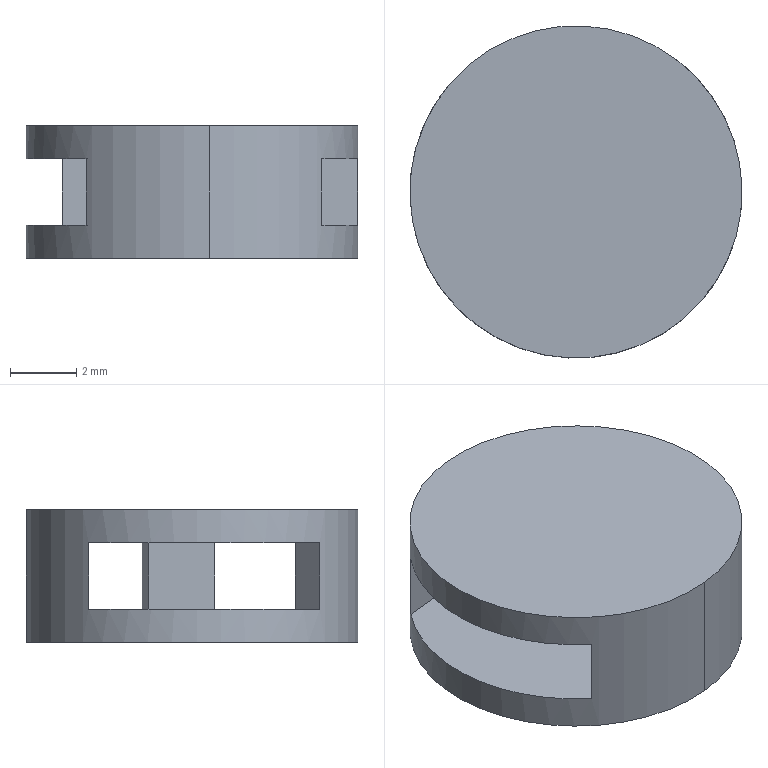Part | SolidWorks | features BaseBody 1 | 1 solid | 11 faces | box 10 x 10 x 4 mm | volume 194.495 mm3 | plane 9 | cylinder 2 | commonest cylinder face diameters 10 x2
STEP:
#1=CARTESIAN_POINT('',(349.672,130.094,60.5));
#2=VERTEX_POINT('',#1);
#3=CARTESIAN_POINT('',(349.672,130.094,62.5));
#4=VERTEX_POINT('',#3);
#5=CARTESIAN_POINT('',(349.672,130.094,63.5));
#6=DIRECTION('',(0.,0.,1.));
#7=VECTOR('',#6,1000.);
#8=LINE('',#5,#7);
#9=EDGE_CURVE('',#2,#4,#8,.T.);
#10=ORIENTED_EDGE('',*,*,#9,.T.);
#11=CARTESIAN_POINT('',(350.393,123.132,62.5));
#12=VERTEX_POINT('',#11);
#13=CARTESIAN_POINT('',(353.585,126.98,62.5));
#14=DIRECTION('',(0.,0.,1.));
#15=DIRECTION('',(-0.1029,0.9947,0.));
#16=AXIS2_PLACEMENT_3D('',#13,#14,#15);
#17=CIRCLE('',#16,5.);
#18=EDGE_CURVE('',#4,#12,#17,.T.);
#19=ORIENTED_EDGE('',*,*,#18,.T.);
#20=CARTESIAN_POINT('',(350.393,123.132,60.5));
#21=VERTEX_POINT('',#20);
#22=CARTESIAN_POINT('',(350.393,123.132,63.5));
#23=DIRECTION('',(0.,0.,-1.));
#24=VECTOR('',#23,1000.);
#25=LINE('',#22,#24);
#26=EDGE_CURVE('',#12,#21,#25,.T.);
#27=ORIENTED_EDGE('',*,*,#26,.T.);
#28=CARTESIAN_POINT('',(353.585,126.98,60.5));
#29=DIRECTION('',(0.,0.,-1.));
#30=DIRECTION('',(0.1029,-0.9947,0.));
#31=AXIS2_PLACEMENT_3D('',#28,#29,#30);
#32=CIRCLE('',#31,5.);
#33=EDGE_CURVE('',#21,#2,#32,.T.);
#34=ORIENTED_EDGE('',*,*,#33,.T.);
#35=EDGE_LOOP('',(#10,#19,#27,#34));
#36=FACE_BOUND('',#35,.T.);
#37=CARTESIAN_POINT('',(353.07,131.954,63.5));
#38=VERTEX_POINT('',#37);
#39=CARTESIAN_POINT('',(354.099,122.007,63.5));
#40=VERTEX_POINT('',#39);
#41=CARTESIAN_POINT('',(353.585,126.98,63.5));
#42=DIRECTION('',(0.,0.,1.));
#43=DIRECTION('',(-0.1029,0.9947,0.));
#44=AXIS2_PLACEMENT_3D('',#41,#42,#43);
#45=CIRCLE('',#44,5.);
#46=EDGE_CURVE('',#38,#40,#45,.T.);
#47=ORIENTED_EDGE('',*,*,#46,.F.);
#48=CARTESIAN_POINT('',(353.07,131.954,59.5));
#49=VERTEX_POINT('',#48);
#50=CARTESIAN_POINT('',(353.07,131.954,63.5));
#51=DIRECTION('',(0.,0.,-1.));
#52=VECTOR('',#51,1000.);
#53=LINE('',#50,#52);
#54=EDGE_CURVE('',#38,#49,#53,.T.);
#55=ORIENTED_EDGE('',*,*,#54,.T.);
#56=CARTESIAN_POINT('',(354.099,122.007,59.5));
#57=VERTEX_POINT('',#56);
#58=CARTESIAN_POINT('',(353.585,126.98,59.5));
#59=DIRECTION('',(0.,0.,1.));
#60=DIRECTION('',(-0.1029,0.9947,0.));
#61=AXIS2_PLACEMENT_3D('',#58,#59,#60);
#62=CIRCLE('',#61,5.);
#63=EDGE_CURVE('',#49,#57,#62,.T.);
#64=ORIENTED_EDGE('',*,*,#63,.T.);
#65=CARTESIAN_POINT('',(354.099,122.007,63.5));
#66=DIRECTION('',(0.,0.,-1.));
#67=VECTOR('',#66,1000.);
#68=LINE('',#65,#67);
#69=EDGE_CURVE('',#40,#57,#68,.T.);
#70=ORIENTED_EDGE('',*,*,#69,.F.);
#71=EDGE_LOOP('',(#47,#55,#64,#70));
#72=FACE_OUTER_BOUND('',#71,.T.);
#73=CARTESIAN_POINT('',(353.585,126.98,63.5));
#74=DIRECTION('',(0.,0.,-1.));
#75=DIRECTION('',(0.1029,-0.9947,0.));
#76=AXIS2_PLACEMENT_3D('',#73,#74,#75);
#77=CYLINDRICAL_SURFACE('',#76,5.);
#78=ADVANCED_FACE('',(#36,#72),#77,.T.);
#79=ORIENTED_EDGE('',*,*,#54,.F.);
#80=CARTESIAN_POINT('',(353.585,126.98,63.5));
#81=DIRECTION('',(0.,0.,1.));
#82=DIRECTION('',(-0.1029,0.9947,0.));
#83=AXIS2_PLACEMENT_3D('',#80,#81,#82);
#84=CIRCLE('',#83,5.);
#85=EDGE_CURVE('',#40,#38,#84,.T.);
#86=ORIENTED_EDGE('',*,*,#85,.F.);
#87=ORIENTED_EDGE('',*,*,#69,.T.);
#88=CARTESIAN_POINT('',(353.585,126.98,59.5));
#89=DIRECTION('',(0.,0.,1.));
#90=DIRECTION('',(-0.1029,0.9947,0.));
#91=AXIS2_PLACEMENT_3D('',#88,#89,#90);
#92=CIRCLE('',#91,5.);
#93=EDGE_CURVE('',#57,#49,#92,.T.);
#94=ORIENTED_EDGE('',*,*,#93,.T.);
#95=EDGE_LOOP('',(#79,#86,#87,#94));
#96=FACE_OUTER_BOUND('',#95,.T.);
#97=CARTESIAN_POINT('',(358.56,126.49,60.5));
#98=VERTEX_POINT('',#97);
#99=CARTESIAN_POINT('',(357.497,123.867,60.5));
#100=VERTEX_POINT('',#99);
#101=CARTESIAN_POINT('',(353.585,126.98,60.5));
#102=DIRECTION('',(0.,0.,-1.));
#103=DIRECTION('',(0.1029,-0.9947,0.));
#104=AXIS2_PLACEMENT_3D('',#101,#102,#103);
#105=CIRCLE('',#104,5.);
#106=EDGE_CURVE('',#98,#100,#105,.T.);
#107=ORIENTED_EDGE('',*,*,#106,.T.);
#108=CARTESIAN_POINT('',(357.497,123.867,62.5));
#109=VERTEX_POINT('',#108);
#110=CARTESIAN_POINT('',(357.497,123.867,63.5));
#111=DIRECTION('',(0.,0.,1.));
#112=VECTOR('',#111,1000.);
#113=LINE('',#110,#112);
#114=EDGE_CURVE('',#100,#109,#113,.T.);
#115=ORIENTED_EDGE('',*,*,#114,.T.);
#116=CARTESIAN_POINT('',(358.56,126.49,62.5));
#117=VERTEX_POINT('',#116);
#118=CARTESIAN_POINT('',(353.585,126.98,62.5));
#119=DIRECTION('',(0.,0.,1.));
#120=DIRECTION('',(-0.1029,0.9947,0.));
#121=AXIS2_PLACEMENT_3D('',#118,#119,#120);
#122=CIRCLE('',#121,5.);
#123=EDGE_CURVE('',#109,#117,#122,.T.);
#124=ORIENTED_EDGE('',*,*,#123,.T.);
#125=CARTESIAN_POINT('',(358.56,126.49,63.5));
#126=DIRECTION('',(0.,0.,-1.));
#127=VECTOR('',#126,1000.);
#128=LINE('',#125,#127);
#129=EDGE_CURVE('',#117,#98,#128,.T.);
#130=ORIENTED_EDGE('',*,*,#129,.T.);
#131=EDGE_LOOP('',(#107,#115,#124,#130));
#132=FACE_BOUND('',#131,.T.);
#133=CARTESIAN_POINT('',(358.355,128.479,62.5));
#134=VERTEX_POINT('',#133);
#135=CARTESIAN_POINT('',(356.776,130.829,62.5));
#136=VERTEX_POINT('',#135);
#137=CARTESIAN_POINT('',(353.585,126.98,62.5));
#138=DIRECTION('',(0.,0.,1.));
#139=DIRECTION('',(-0.1029,0.9947,0.));
#140=AXIS2_PLACEMENT_3D('',#137,#138,#139);
#141=CIRCLE('',#140,5.);
#142=EDGE_CURVE('',#134,#136,#141,.T.);
#143=ORIENTED_EDGE('',*,*,#142,.T.);
#144=CARTESIAN_POINT('',(356.776,130.829,60.5));
#145=VERTEX_POINT('',#144);
#146=CARTESIAN_POINT('',(356.776,130.829,63.5));
#147=DIRECTION('',(0.,0.,-1.));
#148=VECTOR('',#147,1000.);
#149=LINE('',#146,#148);
#150=EDGE_CURVE('',#136,#145,#149,.T.);
#151=ORIENTED_EDGE('',*,*,#150,.T.);
#152=CARTESIAN_POINT('',(358.355,128.479,60.5));
#153=VERTEX_POINT('',#152);
#154=CARTESIAN_POINT('',(353.585,126.98,60.5));
#155=DIRECTION('',(0.,0.,-1.));
#156=DIRECTION('',(0.1029,-0.9947,0.));
#157=AXIS2_PLACEMENT_3D('',#154,#155,#156);
#158=CIRCLE('',#157,5.);
#159=EDGE_CURVE('',#145,#153,#158,.T.);
#160=ORIENTED_EDGE('',*,*,#159,.T.);
#161=CARTESIAN_POINT('',(358.355,128.479,63.5));
#162=DIRECTION('',(0.,0.,1.));
#163=VECTOR('',#162,1000.);
#164=LINE('',#161,#163);
#165=EDGE_CURVE('',#153,#134,#164,.T.);
#166=ORIENTED_EDGE('',*,*,#165,.T.);
#167=EDGE_LOOP('',(#143,#151,#160,#166));
#168=FACE_BOUND('',#167,.T.);
#169=CARTESIAN_POINT('',(353.585,126.98,63.5));
#170=DIRECTION('',(0.,0.,-1.));
#171=DIRECTION('',(0.1029,-0.9947,0.));
#172=AXIS2_PLACEMENT_3D('',#169,#170,#171);
#173=CYLINDRICAL_SURFACE('',#172,5.);
#174=ADVANCED_FACE('',(#96,#132,#168),#173,.T.);
#175=ORIENTED_EDGE('',*,*,#85,.T.);
#176=ORIENTED_EDGE('',*,*,#46,.T.);
#177=EDGE_LOOP('',(#175,#176));
#178=FACE_OUTER_BOUND('',#177,.T.);
#179=CARTESIAN_POINT('',(353.585,126.98,63.5));
#180=DIRECTION('',(0.,0.,1.));
#181=DIRECTION('',(-0.1029,0.9947,0.));
#182=AXIS2_PLACEMENT_3D('',#179,#180,#181);
#183=PLANE('',#182);
#184=ADVANCED_FACE('',(#178),#183,.T.);
#185=ORIENTED_EDGE('',*,*,#93,.F.);
#186=ORIENTED_EDGE('',*,*,#63,.F.);
#187=EDGE_LOOP('',(#185,#186));
#188=FACE_OUTER_BOUND('',#187,.T.);
#189=CARTESIAN_POINT('',(353.585,126.98,59.5));
#190=DIRECTION('',(0.,0.,1.));
#191=DIRECTION('',(-0.1029,0.9947,0.));
#192=AXIS2_PLACEMENT_3D('',#189,#190,#191);
#193=PLANE('',#192);
#194=ADVANCED_FACE('',(#188),#193,.F.);
#195=CARTESIAN_POINT('',(356.929,123.808,62.5));
#196=DIRECTION('',(-0.9947,-0.1029,0.));
#197=VECTOR('',#196,1000.);
#198=LINE('',#195,#197);
#199=EDGE_CURVE('',#109,#12,#198,.T.);
#200=ORIENTED_EDGE('',*,*,#199,.F.);
#201=ORIENTED_EDGE('',*,*,#114,.F.);
#202=CARTESIAN_POINT('',(356.929,123.808,60.5));
#203=DIRECTION('',(-0.9947,-0.1029,0.));
#204=VECTOR('',#203,1000.);
#205=LINE('',#202,#204);
#206=EDGE_CURVE('',#100,#21,#205,.T.);
#207=ORIENTED_EDGE('',*,*,#206,.T.);
#208=ORIENTED_EDGE('',*,*,#26,.F.);
#209=EDGE_LOOP('',(#200,#201,#207,#208));
#210=FACE_OUTER_BOUND('',#209,.T.);
#211=CARTESIAN_POINT('',(356.929,123.808,60.5));
#212=DIRECTION('',(0.1029,-0.9947,0.));
#213=DIRECTION('',(0.,0.,1.));
#214=AXIS2_PLACEMENT_3D('',#211,#212,#213);
#215=PLANE('',#214);
#216=ADVANCED_FACE('',(#210),#215,.F.);
#217=ORIENTED_EDGE('',*,*,#206,.F.);
#218=ORIENTED_EDGE('',*,*,#106,.F.);
#219=CARTESIAN_POINT('',(356.672,126.295,60.5));
#220=VERTEX_POINT('',#219);
#221=CARTESIAN_POINT('',(358.661,126.5,60.5));
#222=DIRECTION('',(-0.9947,-0.1029,0.));
#223=VECTOR('',#222,1000.);
#224=LINE('',#221,#223);
#225=EDGE_CURVE('',#98,#220,#224,.T.);
#226=ORIENTED_EDGE('',*,*,#225,.T.);
#227=CARTESIAN_POINT('',(356.466,128.284,60.5));
#228=VERTEX_POINT('',#227);
#229=CARTESIAN_POINT('',(356.929,123.808,60.5));
#230=DIRECTION('',(0.1029,-0.9947,0.));
#231=VECTOR('',#230,1000.);
#232=LINE('',#229,#231);
#233=EDGE_CURVE('',#228,#220,#232,.T.);
#234=ORIENTED_EDGE('',*,*,#233,.F.);
#235=CARTESIAN_POINT('',(358.455,128.49,60.5));
#236=DIRECTION('',(-0.9947,-0.1029,0.));
#237=VECTOR('',#236,1000.);
#238=LINE('',#235,#237);
#239=EDGE_CURVE('',#153,#228,#238,.T.);
#240=ORIENTED_EDGE('',*,*,#239,.F.);
#241=ORIENTED_EDGE('',*,*,#159,.F.);
#242=CARTESIAN_POINT('',(356.208,130.771,60.5));
#243=DIRECTION('',(-0.9947,-0.1029,0.));
#244=VECTOR('',#243,1000.);
#245=LINE('',#242,#244);
#246=EDGE_CURVE('',#145,#2,#245,.T.);
#247=ORIENTED_EDGE('',*,*,#246,.T.);
#248=ORIENTED_EDGE('',*,*,#33,.F.);
#249=EDGE_LOOP('',(#217,#218,#226,#234,#240,#241,#247,#248));
#250=FACE_OUTER_BOUND('',#249,.T.);
#251=CARTESIAN_POINT('',(356.929,123.808,60.5));
#252=DIRECTION('',(0.,0.,-1.));
#253=DIRECTION('',(0.1029,-0.9947,0.));
#254=AXIS2_PLACEMENT_3D('',#251,#252,#253);
#255=PLANE('',#254);
#256=ADVANCED_FACE('',(#250),#255,.F.);
#257=ORIENTED_EDGE('',*,*,#246,.F.);
#258=ORIENTED_EDGE('',*,*,#150,.F.);
#259=CARTESIAN_POINT('',(356.208,130.771,62.5));
#260=DIRECTION('',(-0.9947,-0.1029,0.));
#261=VECTOR('',#260,1000.);
#262=LINE('',#259,#261);
#263=EDGE_CURVE('',#136,#4,#262,.T.);
#264=ORIENTED_EDGE('',*,*,#263,.T.);
#265=ORIENTED_EDGE('',*,*,#9,.F.);
#266=EDGE_LOOP('',(#257,#258,#264,#265));
#267=FACE_OUTER_BOUND('',#266,.T.);
#268=CARTESIAN_POINT('',(356.208,130.771,60.5));
#269=DIRECTION('',(-0.1029,0.9947,0.));
#270=DIRECTION('',(0.,0.,-1.));
#271=AXIS2_PLACEMENT_3D('',#268,#269,#270);
#272=PLANE('',#271);
#273=ADVANCED_FACE('',(#267),#272,.F.);
#274=ORIENTED_EDGE('',*,*,#263,.F.);
#275=ORIENTED_EDGE('',*,*,#142,.F.);
#276=CARTESIAN_POINT('',(356.466,128.284,62.5));
#277=VERTEX_POINT('',#276);
#278=CARTESIAN_POINT('',(358.455,128.49,62.5));
#279=DIRECTION('',(-0.9947,-0.1029,0.));
#280=VECTOR('',#279,1000.);
#281=LINE('',#278,#280);
#282=EDGE_CURVE('',#134,#277,#281,.T.);
#283=ORIENTED_EDGE('',*,*,#282,.T.);
#284=CARTESIAN_POINT('',(356.672,126.295,62.5));
#285=VERTEX_POINT('',#284);
#286=CARTESIAN_POINT('',(356.929,123.808,62.5));
#287=DIRECTION('',(-0.1029,0.9947,0.));
#288=VECTOR('',#287,1000.);
#289=LINE('',#286,#288);
#290=EDGE_CURVE('',#285,#277,#289,.T.);
#291=ORIENTED_EDGE('',*,*,#290,.F.);
#292=CARTESIAN_POINT('',(358.661,126.5,62.5));
#293=DIRECTION('',(-0.9947,-0.1029,0.));
#294=VECTOR('',#293,1000.);
#295=LINE('',#292,#294);
#296=EDGE_CURVE('',#117,#285,#295,.T.);
#297=ORIENTED_EDGE('',*,*,#296,.F.);
#298=ORIENTED_EDGE('',*,*,#123,.F.);
#299=ORIENTED_EDGE('',*,*,#199,.T.);
#300=ORIENTED_EDGE('',*,*,#18,.F.);
#301=EDGE_LOOP('',(#274,#275,#283,#291,#297,#298,#299,#300));
#302=FACE_OUTER_BOUND('',#301,.T.);
#303=CARTESIAN_POINT('',(356.929,123.808,62.5));
#304=DIRECTION('',(0.,0.,1.));
#305=DIRECTION('',(-0.1029,0.9947,0.));
#306=AXIS2_PLACEMENT_3D('',#303,#304,#305);
#307=PLANE('',#306);
#308=ADVANCED_FACE('',(#302),#307,.F.);
#309=CARTESIAN_POINT('',(356.672,126.295,60.5));
#310=DIRECTION('',(0.,0.,-1.));
#311=VECTOR('',#310,1000.);
#312=LINE('',#309,#311);
#313=EDGE_CURVE('',#285,#220,#312,.T.);
#314=ORIENTED_EDGE('',*,*,#313,.F.);
#315=ORIENTED_EDGE('',*,*,#290,.T.);
#316=CARTESIAN_POINT('',(356.466,128.284,60.5));
#317=DIRECTION('',(0.,0.,1.));
#318=VECTOR('',#317,1000.);
#319=LINE('',#316,#318);
#320=EDGE_CURVE('',#228,#277,#319,.T.);
#321=ORIENTED_EDGE('',*,*,#320,.F.);
#322=ORIENTED_EDGE('',*,*,#233,.T.);
#323=EDGE_LOOP('',(#314,#315,#321,#322));
#324=FACE_OUTER_BOUND('',#323,.T.);
#325=CARTESIAN_POINT('',(356.929,123.808,62.5));
#326=DIRECTION('',(-0.9947,-0.1029,0.));
#327=DIRECTION('',(0.,0.,1.));
#328=AXIS2_PLACEMENT_3D('',#325,#326,#327);
#329=PLANE('',#328);
#330=ADVANCED_FACE('',(#324),#329,.T.);
#331=ORIENTED_EDGE('',*,*,#239,.T.);
#332=ORIENTED_EDGE('',*,*,#320,.T.);
#333=ORIENTED_EDGE('',*,*,#282,.F.);
#334=ORIENTED_EDGE('',*,*,#165,.F.);
#335=EDGE_LOOP('',(#331,#332,#333,#334));
#336=FACE_OUTER_BOUND('',#335,.T.);
#337=CARTESIAN_POINT('',(358.455,128.49,60.5));
#338=DIRECTION('',(0.1029,-0.9947,0.));
#339=DIRECTION('',(0.,0.,1.));
#340=AXIS2_PLACEMENT_3D('',#337,#338,#339);
#341=PLANE('',#340);
#342=ADVANCED_FACE('',(#336),#341,.F.);
#343=ORIENTED_EDGE('',*,*,#296,.T.);
#344=ORIENTED_EDGE('',*,*,#313,.T.);
#345=ORIENTED_EDGE('',*,*,#225,.F.);
#346=ORIENTED_EDGE('',*,*,#129,.F.);
#347=EDGE_LOOP('',(#343,#344,#345,#346));
#348=FACE_OUTER_BOUND('',#347,.T.);
#349=CARTESIAN_POINT('',(358.661,126.5,60.5));
#350=DIRECTION('',(-0.1029,0.9947,0.));
#351=DIRECTION('',(0.,0.,-1.));
#352=AXIS2_PLACEMENT_3D('',#349,#350,#351);
#353=PLANE('',#352);
#354=ADVANCED_FACE('',(#348),#353,.F.);
#355=CLOSED_SHELL('',(#78,#174,#184,#194,#216,#256,#273,#308,#330,#342,#354));
#356=MANIFOLD_SOLID_BREP('',#355);
#357=CARTESIAN_POINT('',(0.,0.,0.));
#358=DIRECTION('',(0.,0.,1.));
#359=DIRECTION('',(1.,0.,0.));
#360=AXIS2_PLACEMENT_3D('',#357,#358,#359);
#361=(LENGTH_UNIT()NAMED_UNIT(*)SI_UNIT(.MILLI.,.METRE.));
#362=UNCERTAINTY_MEASURE_WITH_UNIT(LENGTH_MEASURE(0.00001),#361,'','');
#363=(NAMED_UNIT(*)PLANE_ANGLE_UNIT()SI_UNIT($,.RADIAN.));
#364=(NAMED_UNIT(*)SI_UNIT($,.STERADIAN.)SOLID_ANGLE_UNIT());
#365=(GEOMETRIC_REPRESENTATION_CONTEXT(3)GLOBAL_UNCERTAINTY_ASSIGNED_CONTEXT((#362))GLOBAL_UNIT_ASSIGNED_CONTEXT((#361,#363,#364))REPRESENTATION_CONTEXT('',''));
#366=ADVANCED_BREP_SHAPE_REPRESENTATION('',(#356,#360),#365);